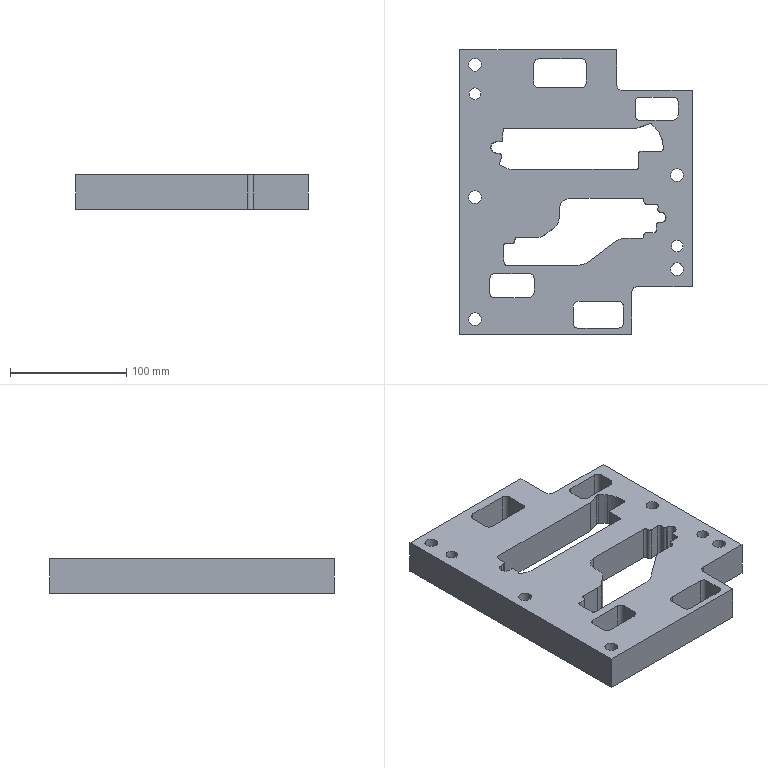Part | STEP file | 212_id658_x_t | 1 solid | 130 faces | box 200 x 245 x 30 mm | volume 915003 mm3 | cylinder 53 | plane 52 | other 22 | spline 3 | commonest cylinder face diameters 4 x15 8 x12 10 x8 11 x7 17 x5 20 x5